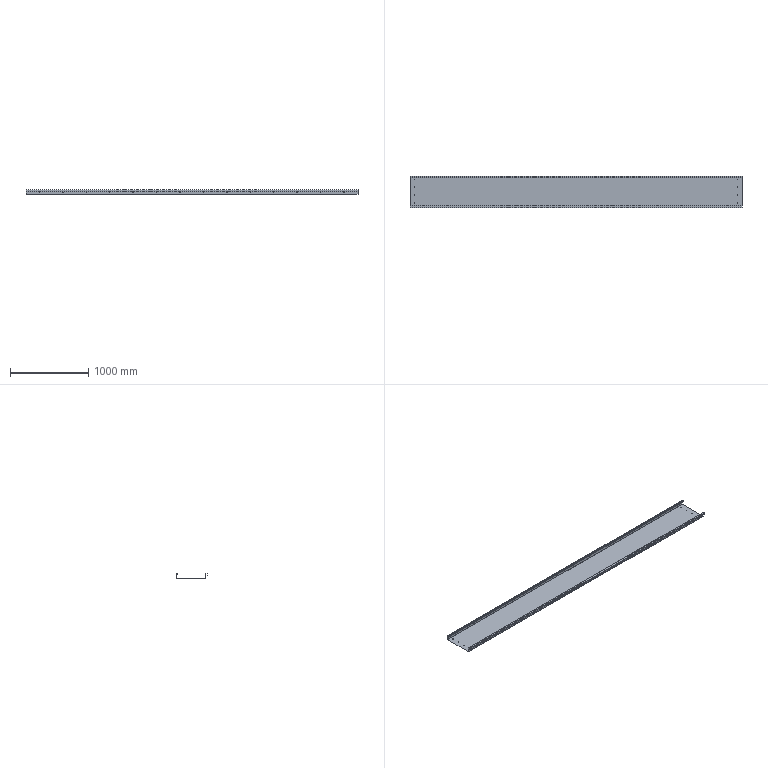Part | STEP file | TS-S90 | 1 solid | 126 faces | box 4250 x 403 x 62 mm | volume 4816834 mm3 | cylinder 84 | plane 42 | commonest cylinder face diameters 5.4 x56 7 x16 0.4 x6 4.4 x6